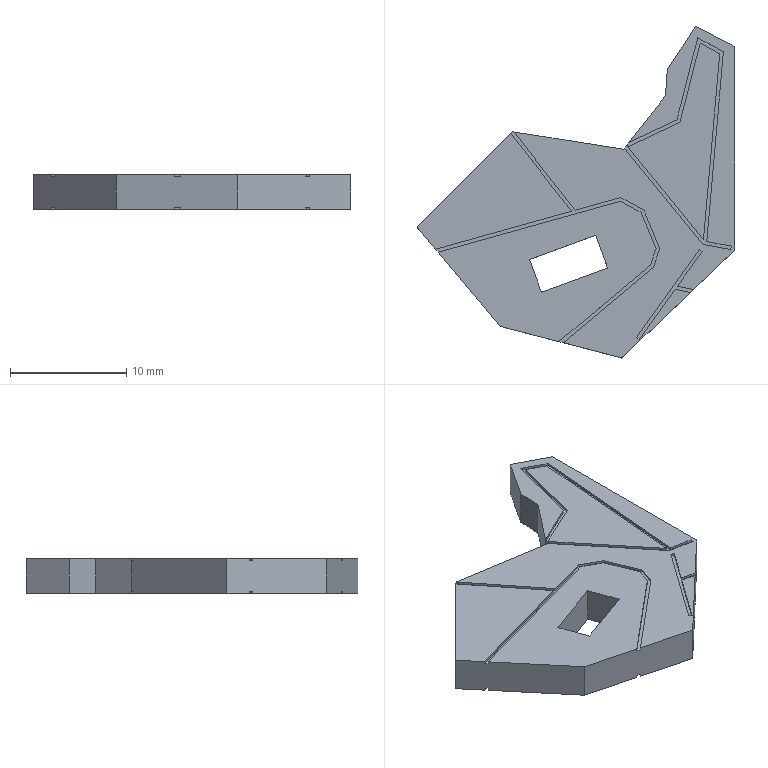Part | SolidWorks | features BaseBody 1 | 1 solid | 102 faces | box 27.356 x 28.569 x 3 mm | volume 1227 mm3 | plane 94 | spline 8